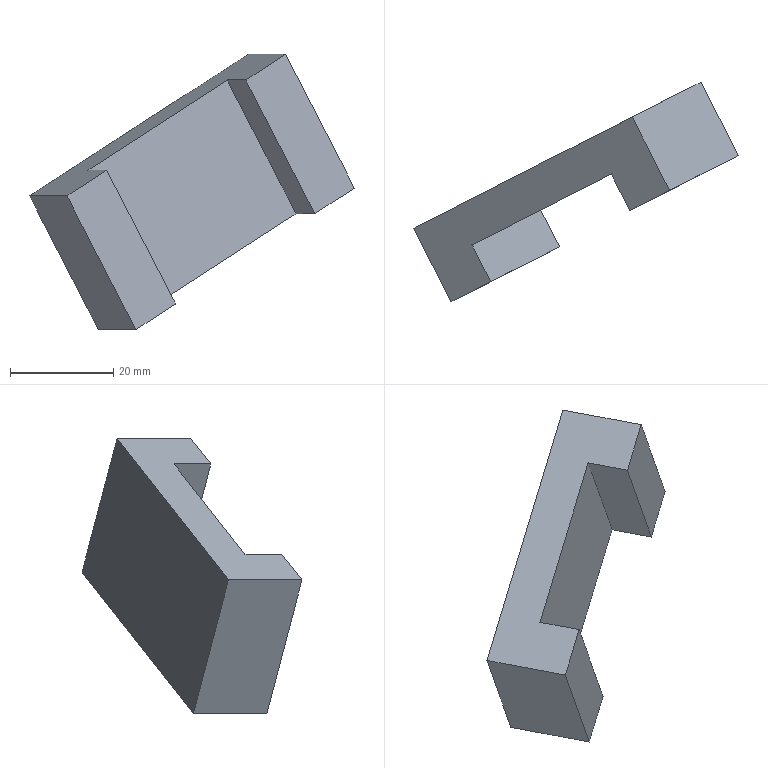Part | NX | features solid 2 | 1 solid | 10 faces | box 63.069 x 42.69 x 53.481 mm | volume 18000 mm3 | plane 10
STEP:
#1=CARTESIAN_POINT('',(-1663.59,-424.525,66.147));
#2=VERTEX_POINT('',#1);
#3=CARTESIAN_POINT('',(-1667.222,-417.397,66.147));
#4=VERTEX_POINT('',#3);
#5=CARTESIAN_POINT('',(-1663.59,-424.525,66.147));
#6=DIRECTION('',(-0.454,0.891,0.));
#7=VECTOR('',#6,1000.);
#8=LINE('',#5,#7);
#9=EDGE_CURVE('',#2,#4,#8,.T.);
#10=ORIENTED_EDGE('',*,*,#9,.T.);
#11=CARTESIAN_POINT('',(-1680.587,-424.206,92.128));
#12=VERTEX_POINT('',#11);
#13=CARTESIAN_POINT('',(-1680.587,-424.206,92.128));
#14=DIRECTION('',(0.4455,0.227,-0.866));
#15=VECTOR('',#14,1000.);
#16=LINE('',#13,#15);
#17=EDGE_CURVE('',#12,#4,#16,.T.);
#18=ORIENTED_EDGE('',*,*,#17,.F.);
#19=CARTESIAN_POINT('',(-1676.955,-431.334,92.128));
#20=VERTEX_POINT('',#19);
#21=CARTESIAN_POINT('',(-1676.955,-431.334,92.128));
#22=DIRECTION('',(-0.454,0.891,0.));
#23=VECTOR('',#22,1000.);
#24=LINE('',#21,#23);
#25=EDGE_CURVE('',#20,#12,#24,.T.);
#26=ORIENTED_EDGE('',*,*,#25,.F.);
#27=CARTESIAN_POINT('',(-1676.955,-431.334,92.128));
#28=DIRECTION('',(0.4455,0.227,-0.866));
#29=VECTOR('',#28,1000.);
#30=LINE('',#27,#29);
#31=EDGE_CURVE('',#20,#2,#30,.T.);
#32=ORIENTED_EDGE('',*,*,#31,.T.);
#33=EDGE_LOOP('',(#10,#18,#26,#32));
#34=FACE_BOUND('',#33,.T.);
#35=CARTESIAN_POINT('',(-1676.955,-431.334,92.128));
#36=DIRECTION('',(0.7716,0.3932,0.5));
#37=DIRECTION('',(0.4455,0.227,-0.866));
#38=AXIS2_PLACEMENT_3D('',#35,#36,#37);
#39=PLANE('',#38);
#40=ADVANCED_FACE('',(#34),#39,.T.);
#41=CARTESIAN_POINT('',(-1640.215,-403.636,83.647));
#42=VERTEX_POINT('',#41);
#43=CARTESIAN_POINT('',(-1667.222,-417.397,66.147));
#44=DIRECTION('',(0.7716,0.3932,0.5));
#45=VECTOR('',#44,1000.);
#46=LINE('',#43,#45);
#47=EDGE_CURVE('',#4,#42,#46,.T.);
#48=ORIENTED_EDGE('',*,*,#47,.T.);
#49=CARTESIAN_POINT('',(-1653.58,-410.446,109.628));
#50=VERTEX_POINT('',#49);
#51=CARTESIAN_POINT('',(-1653.58,-410.446,109.628));
#52=DIRECTION('',(0.4455,0.227,-0.866));
#53=VECTOR('',#52,1000.);
#54=LINE('',#51,#53);
#55=EDGE_CURVE('',#50,#42,#54,.T.);
#56=ORIENTED_EDGE('',*,*,#55,.F.);
#57=CARTESIAN_POINT('',(-1680.587,-424.206,92.128));
#58=DIRECTION('',(0.7716,0.3932,0.5));
#59=VECTOR('',#58,1000.);
#60=LINE('',#57,#59);
#61=EDGE_CURVE('',#12,#50,#60,.T.);
#62=ORIENTED_EDGE('',*,*,#61,.F.);
#63=ORIENTED_EDGE('',*,*,#17,.T.);
#64=EDGE_LOOP('',(#48,#56,#62,#63));
#65=FACE_BOUND('',#64,.T.);
#66=CARTESIAN_POINT('',(-1680.587,-424.206,92.128));
#67=DIRECTION('',(0.454,-0.891,0.));
#68=DIRECTION('',(0.,0.,1.));
#69=AXIS2_PLACEMENT_3D('',#66,#67,#68);
#70=PLANE('',#69);
#71=ADVANCED_FACE('',(#65),#70,.T.);
#72=CARTESIAN_POINT('',(-1636.583,-410.764,83.647));
#73=VERTEX_POINT('',#72);
#74=CARTESIAN_POINT('',(-1636.583,-410.764,83.647));
#75=DIRECTION('',(-0.454,0.891,0.));
#76=VECTOR('',#75,1000.);
#77=LINE('',#74,#76);
#78=EDGE_CURVE('',#73,#42,#77,.T.);
#79=ORIENTED_EDGE('',*,*,#78,.F.);
#80=CARTESIAN_POINT('',(-1649.948,-417.574,109.628));
#81=VERTEX_POINT('',#80);
#82=CARTESIAN_POINT('',(-1649.948,-417.574,109.628));
#83=DIRECTION('',(0.4455,0.227,-0.866));
#84=VECTOR('',#83,1000.);
#85=LINE('',#82,#84);
#86=EDGE_CURVE('',#81,#73,#85,.T.);
#87=ORIENTED_EDGE('',*,*,#86,.F.);
#88=CARTESIAN_POINT('',(-1649.948,-417.574,109.628));
#89=DIRECTION('',(-0.454,0.891,0.));
#90=VECTOR('',#89,1000.);
#91=LINE('',#88,#90);
#92=EDGE_CURVE('',#81,#50,#91,.T.);
#93=ORIENTED_EDGE('',*,*,#92,.T.);
#94=ORIENTED_EDGE('',*,*,#55,.T.);
#95=EDGE_LOOP('',(#79,#87,#93,#94));
#96=FACE_BOUND('',#95,.T.);
#97=CARTESIAN_POINT('',(-1649.948,-417.574,109.628));
#98=DIRECTION('',(0.7716,0.3932,0.5));
#99=DIRECTION('',(0.4455,0.227,-0.866));
#100=AXIS2_PLACEMENT_3D('',#97,#98,#99);
#101=PLANE('',#100);
#102=ADVANCED_FACE('',(#96),#101,.F.);
#103=CARTESIAN_POINT('',(-1628.867,-406.832,88.647));
#104=VERTEX_POINT('',#103);
#105=CARTESIAN_POINT('',(-1628.867,-406.832,88.647));
#106=DIRECTION('',(-0.7716,-0.3932,-0.5));
#107=VECTOR('',#106,1000.);
#108=LINE('',#105,#107);
#109=EDGE_CURVE('',#104,#73,#108,.T.);
#110=ORIENTED_EDGE('',*,*,#109,.F.);
#111=CARTESIAN_POINT('',(-1642.232,-413.642,114.628));
#112=VERTEX_POINT('',#111);
#113=CARTESIAN_POINT('',(-1642.232,-413.642,114.628));
#114=DIRECTION('',(0.4455,0.227,-0.866));
#115=VECTOR('',#114,1000.);
#116=LINE('',#113,#115);
#117=EDGE_CURVE('',#112,#104,#116,.T.);
#118=ORIENTED_EDGE('',*,*,#117,.F.);
#119=CARTESIAN_POINT('',(-1642.232,-413.642,114.628));
#120=DIRECTION('',(-0.7716,-0.3932,-0.5));
#121=VECTOR('',#120,1000.);
#122=LINE('',#119,#121);
#123=EDGE_CURVE('',#112,#81,#122,.T.);
#124=ORIENTED_EDGE('',*,*,#123,.T.);
#125=ORIENTED_EDGE('',*,*,#86,.T.);
#126=EDGE_LOOP('',(#110,#118,#124,#125));
#127=FACE_BOUND('',#126,.T.);
#128=CARTESIAN_POINT('',(-1642.232,-413.642,114.628));
#129=DIRECTION('',(-0.454,0.891,0.));
#130=DIRECTION('',(0.,0.,-1.));
#131=AXIS2_PLACEMENT_3D('',#128,#129,#130);
#132=PLANE('',#131);
#133=ADVANCED_FACE('',(#127),#132,.F.);
#134=CARTESIAN_POINT('',(-1636.131,-392.576,88.647));
#135=VERTEX_POINT('',#134);
#136=CARTESIAN_POINT('',(-1628.867,-406.832,88.647));
#137=DIRECTION('',(-0.454,0.891,0.));
#138=VECTOR('',#137,1000.);
#139=LINE('',#136,#138);
#140=EDGE_CURVE('',#104,#135,#139,.T.);
#141=ORIENTED_EDGE('',*,*,#140,.T.);
#142=CARTESIAN_POINT('',(-1649.496,-399.386,114.628));
#143=VERTEX_POINT('',#142);
#144=CARTESIAN_POINT('',(-1649.496,-399.386,114.628));
#145=DIRECTION('',(0.4455,0.227,-0.866));
#146=VECTOR('',#145,1000.);
#147=LINE('',#144,#146);
#148=EDGE_CURVE('',#143,#135,#147,.T.);
#149=ORIENTED_EDGE('',*,*,#148,.F.);
#150=CARTESIAN_POINT('',(-1642.232,-413.642,114.628));
#151=DIRECTION('',(-0.454,0.891,0.));
#152=VECTOR('',#151,1000.);
#153=LINE('',#150,#152);
#154=EDGE_CURVE('',#112,#143,#153,.T.);
#155=ORIENTED_EDGE('',*,*,#154,.F.);
#156=ORIENTED_EDGE('',*,*,#117,.T.);
#157=EDGE_LOOP('',(#141,#149,#155,#156));
#158=FACE_BOUND('',#157,.T.);
#159=CARTESIAN_POINT('',(-1642.232,-413.642,114.628));
#160=DIRECTION('',(0.7716,0.3932,0.5));
#161=DIRECTION('',(0.4455,0.227,-0.866));
#162=AXIS2_PLACEMENT_3D('',#159,#160,#161);
#163=PLANE('',#162);
#164=ADVANCED_FACE('',(#158),#163,.T.);
#165=CARTESIAN_POINT('',(-1678.571,-414.2,61.147));
#166=VERTEX_POINT('',#165);
#167=CARTESIAN_POINT('',(-1636.131,-392.576,88.647));
#168=DIRECTION('',(-0.7716,-0.3932,-0.5));
#169=VECTOR('',#168,1000.);
#170=LINE('',#167,#169);
#171=EDGE_CURVE('',#135,#166,#170,.T.);
#172=ORIENTED_EDGE('',*,*,#171,.T.);
#173=CARTESIAN_POINT('',(-1691.936,-421.01,87.128));
#174=VERTEX_POINT('',#173);
#175=CARTESIAN_POINT('',(-1691.936,-421.01,87.128));
#176=DIRECTION('',(0.4455,0.227,-0.866));
#177=VECTOR('',#176,1000.);
#178=LINE('',#175,#177);
#179=EDGE_CURVE('',#174,#166,#178,.T.);
#180=ORIENTED_EDGE('',*,*,#179,.F.);
#181=CARTESIAN_POINT('',(-1649.496,-399.386,114.628));
#182=DIRECTION('',(-0.7716,-0.3932,-0.5));
#183=VECTOR('',#182,1000.);
#184=LINE('',#181,#183);
#185=EDGE_CURVE('',#143,#174,#184,.T.);
#186=ORIENTED_EDGE('',*,*,#185,.F.);
#187=ORIENTED_EDGE('',*,*,#148,.T.);
#188=EDGE_LOOP('',(#172,#180,#186,#187));
#189=FACE_BOUND('',#188,.T.);
#190=CARTESIAN_POINT('',(-1649.496,-399.386,114.628));
#191=DIRECTION('',(-0.454,0.891,0.));
#192=DIRECTION('',(0.,0.,-1.));
#193=AXIS2_PLACEMENT_3D('',#190,#191,#192);
#194=PLANE('',#193);
#195=ADVANCED_FACE('',(#189),#194,.T.);
#196=CARTESIAN_POINT('',(-1671.307,-428.456,61.147));
#197=VERTEX_POINT('',#196);
#198=CARTESIAN_POINT('',(-1678.571,-414.2,61.147));
#199=DIRECTION('',(0.454,-0.891,0.));
#200=VECTOR('',#199,1000.);
#201=LINE('',#198,#200);
#202=EDGE_CURVE('',#166,#197,#201,.T.);
#203=ORIENTED_EDGE('',*,*,#202,.T.);
#204=CARTESIAN_POINT('',(-1684.672,-435.266,87.128));
#205=VERTEX_POINT('',#204);
#206=CARTESIAN_POINT('',(-1684.672,-435.266,87.128));
#207=DIRECTION('',(0.4455,0.227,-0.866));
#208=VECTOR('',#207,1000.);
#209=LINE('',#206,#208);
#210=EDGE_CURVE('',#205,#197,#209,.T.);
#211=ORIENTED_EDGE('',*,*,#210,.F.);
#212=CARTESIAN_POINT('',(-1691.936,-421.01,87.128));
#213=DIRECTION('',(0.454,-0.891,0.));
#214=VECTOR('',#213,1000.);
#215=LINE('',#212,#214);
#216=EDGE_CURVE('',#174,#205,#215,.T.);
#217=ORIENTED_EDGE('',*,*,#216,.F.);
#218=ORIENTED_EDGE('',*,*,#179,.T.);
#219=EDGE_LOOP('',(#203,#211,#217,#218));
#220=FACE_BOUND('',#219,.T.);
#221=CARTESIAN_POINT('',(-1691.936,-421.01,87.128));
#222=DIRECTION('',(-0.7716,-0.3932,-0.5));
#223=DIRECTION('',(-0.4455,-0.227,0.866));
#224=AXIS2_PLACEMENT_3D('',#221,#222,#223);
#225=PLANE('',#224);
#226=ADVANCED_FACE('',(#220),#225,.T.);
#227=CARTESIAN_POINT('',(-1663.59,-424.525,66.147));
#228=DIRECTION('',(-0.7716,-0.3932,-0.5));
#229=VECTOR('',#228,1000.);
#230=LINE('',#227,#229);
#231=EDGE_CURVE('',#2,#197,#230,.T.);
#232=ORIENTED_EDGE('',*,*,#231,.F.);
#233=ORIENTED_EDGE('',*,*,#31,.F.);
#234=CARTESIAN_POINT('',(-1676.955,-431.334,92.128));
#235=DIRECTION('',(-0.7716,-0.3932,-0.5));
#236=VECTOR('',#235,1000.);
#237=LINE('',#234,#236);
#238=EDGE_CURVE('',#20,#205,#237,.T.);
#239=ORIENTED_EDGE('',*,*,#238,.T.);
#240=ORIENTED_EDGE('',*,*,#210,.T.);
#241=EDGE_LOOP('',(#232,#233,#239,#240));
#242=FACE_BOUND('',#241,.T.);
#243=CARTESIAN_POINT('',(-1676.955,-431.334,92.128));
#244=DIRECTION('',(-0.454,0.891,0.));
#245=DIRECTION('',(0.,0.,-1.));
#246=AXIS2_PLACEMENT_3D('',#243,#244,#245);
#247=PLANE('',#246);
#248=ADVANCED_FACE('',(#242),#247,.F.);
#249=ORIENTED_EDGE('',*,*,#25,.T.);
#250=ORIENTED_EDGE('',*,*,#61,.T.);
#251=ORIENTED_EDGE('',*,*,#92,.F.);
#252=ORIENTED_EDGE('',*,*,#123,.F.);
#253=ORIENTED_EDGE('',*,*,#154,.T.);
#254=ORIENTED_EDGE('',*,*,#185,.T.);
#255=ORIENTED_EDGE('',*,*,#216,.T.);
#256=ORIENTED_EDGE('',*,*,#238,.F.);
#257=EDGE_LOOP('',(#249,#250,#251,#252,#253,#254,#255,#256));
#258=FACE_BOUND('',#257,.T.);
#259=CARTESIAN_POINT('',(-1680.587,-424.206,92.128));
#260=DIRECTION('',(-0.4455,-0.227,0.866));
#261=DIRECTION('',(0.7716,0.3932,0.5));
#262=AXIS2_PLACEMENT_3D('',#259,#260,#261);
#263=PLANE('',#262);
#264=ADVANCED_FACE('',(#258),#263,.T.);
#265=ORIENTED_EDGE('',*,*,#9,.F.);
#266=ORIENTED_EDGE('',*,*,#231,.T.);
#267=ORIENTED_EDGE('',*,*,#202,.F.);
#268=ORIENTED_EDGE('',*,*,#171,.F.);
#269=ORIENTED_EDGE('',*,*,#140,.F.);
#270=ORIENTED_EDGE('',*,*,#109,.T.);
#271=ORIENTED_EDGE('',*,*,#78,.T.);
#272=ORIENTED_EDGE('',*,*,#47,.F.);
#273=EDGE_LOOP('',(#265,#266,#267,#268,#269,#270,#271,#272));
#274=FACE_BOUND('',#273,.T.);
#275=CARTESIAN_POINT('',(-1667.222,-417.397,66.147));
#276=DIRECTION('',(-0.4455,-0.227,0.866));
#277=DIRECTION('',(0.7716,0.3932,0.5));
#278=AXIS2_PLACEMENT_3D('',#275,#276,#277);
#279=PLANE('',#278);
#280=ADVANCED_FACE('',(#274),#279,.F.);
#281=CLOSED_SHELL('',(#40,#71,#102,#133,#164,#195,#226,#248,#264,#280));
#282=MANIFOLD_SOLID_BREP('',#281);
#283=(LENGTH_UNIT()NAMED_UNIT(*)SI_UNIT(.MILLI.,.METRE.));
#284=UNCERTAINTY_MEASURE_WITH_UNIT(LENGTH_MEASURE(0.00001),#283,'','');
#285=(NAMED_UNIT(*)PLANE_ANGLE_UNIT()SI_UNIT($,.RADIAN.));
#286=(NAMED_UNIT(*)SI_UNIT($,.STERADIAN.)SOLID_ANGLE_UNIT());
#287=(GEOMETRIC_REPRESENTATION_CONTEXT(3)GLOBAL_UNCERTAINTY_ASSIGNED_CONTEXT((#284))GLOBAL_UNIT_ASSIGNED_CONTEXT((#283,#285,#286))REPRESENTATION_CONTEXT('',''));
#288=ADVANCED_BREP_SHAPE_REPRESENTATION('',(#282),#287);